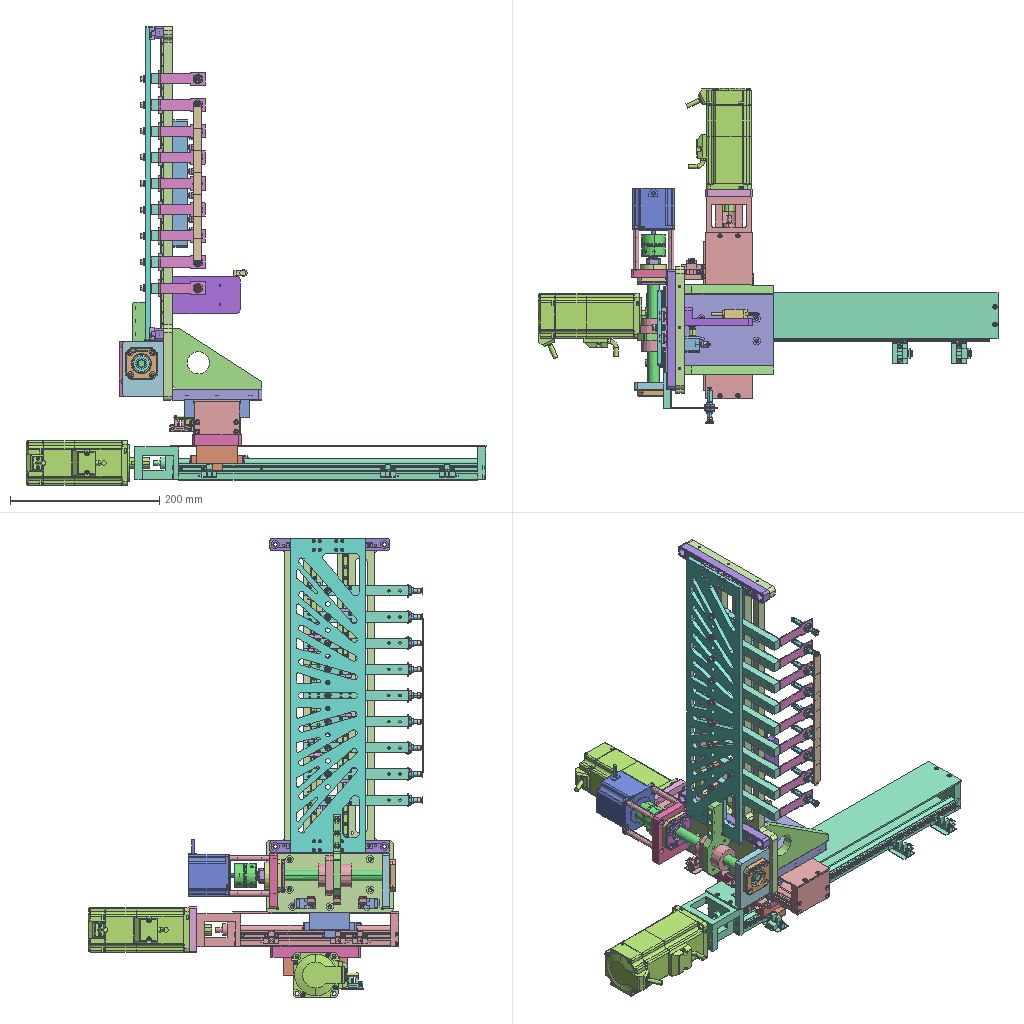Assembly | STEP file | 54 different items | 180 placed | box 616 x 450 x 614 mm
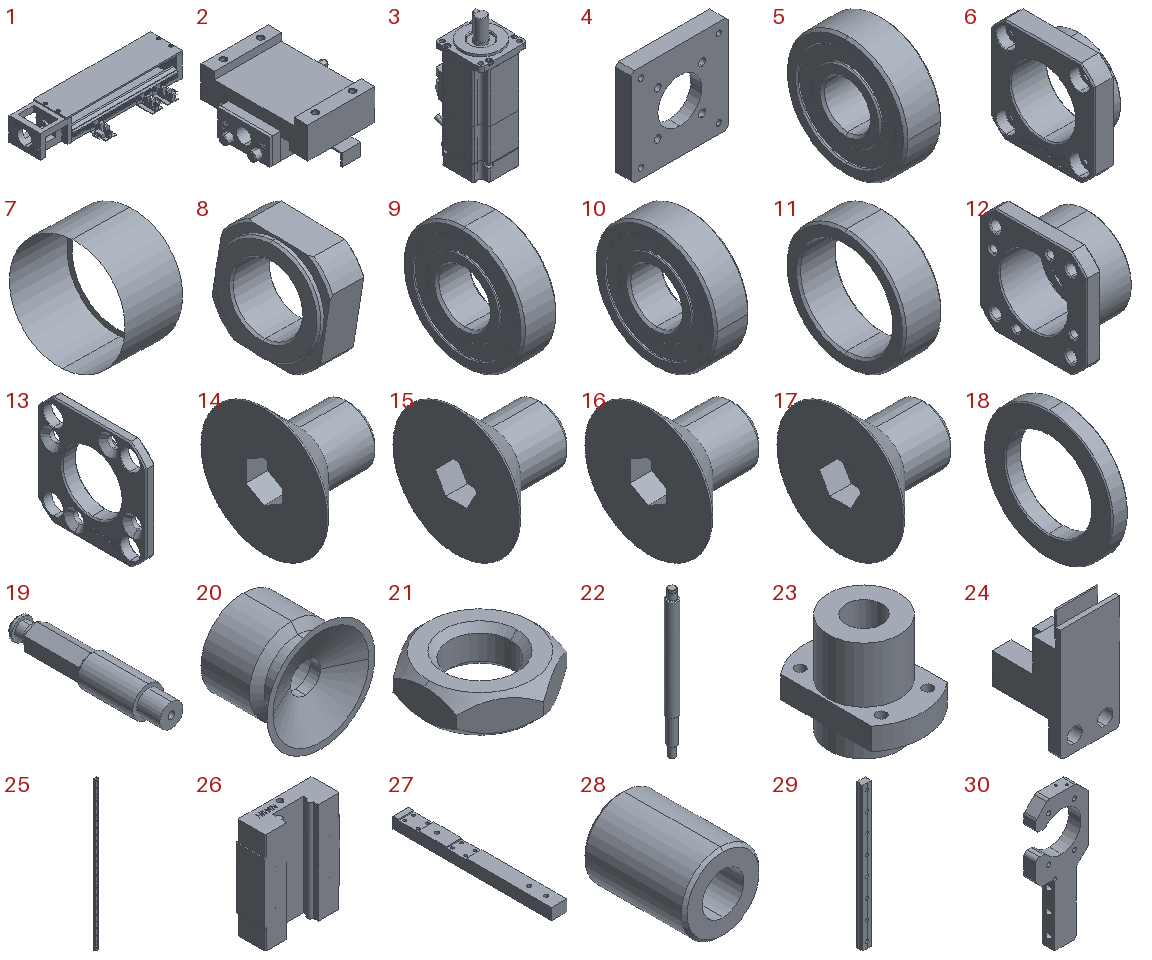Parts list (item | name | quantity | parent item | size | volume):
1 | PRODUCT_ID_1-C-F0-200 | x1 | in KK6005C-200A1-F0CS1-HiwinCorporation-07-20-2018 | 270.02 x 94.86 x 47 mm | 309343 mm3
2 | PRODUCT_ID_2-C-F0-200 | x1 | in KK6005C-200A1-F0CS1-HiwinCorporation-07-20-2018 | 83.5 x 94 x 36 mm | 123650 mm3
3 | C20604RS(Delta 400W) Servo Motor | x2 | in KK6005C-200A1-F0CS1-HiwinCorporation-07-20-2018, KK6010C-400A1-F0CS1-HiwinCorporation-07-20-2018 | 60 x 87.491 x 165.5 mm | 457978 mm3
4 | KK60-F2E KK60 200W Flange Adapter | x1 | in KK6005C-200A1-F0CS1-HiwinCorporation-07-20-2018 | 62 x 10 x 62 mm | 27303 mm3
5 | 6000ZZ-1 | x1 | in LKFF12 | 8 x 26 x 26 mm | 3377 mm3
6 | LFF12-1-1 | x1 | in LKFF12 | 15 x 42 x 42 mm | 10904 mm3
7 | Lock nut 19X8X12 | x1 | in 7 | - | -
8 | Lock nut 19X8X12-1 | x1 | in 7 | 10.153 x 20.245 x 20.375 mm | 1688 mm3
9 | 7001-1 | x1 | in LKFK12 | 8 x 28 x 28 mm | 3796 mm3
10 | 7001_1-1 | x1 | in LKFK12 | 8 x 28 x 28 mm | 3796 mm3
11 | Spacer ring 15-5-12-1 | x1 | in LKFK12 | 5 x 15.5 x 15.5 mm | 371.674 mm3
12 | LFK12-1 | x1 | in LKFK12 | 23 x 44 x 44 mm | 14384 mm3
13 | LFK12-MOD-1 | x1 | in LKFK12 | 6 x 44 x 44 mm | 4397 mm3
14 | M4-6-1 | x1 | in LKFK12 | 6 x 8.819 x 8.819 mm | 121.278 mm3
15 | M4-6_1-1 | x1 | in LKFK12 | 6 x 8.819 x 8.819 mm | 121.278 mm3
16 | M4-6_2-1 | x1 | in LKFK12 | 6 x 8.819 x 8.819 mm | 121.278 mm3
17 | M4-6_3-1 | x1 | in LKFK12 | 6 x 8.819 x 8.819 mm | 121.278 mm3
18 | Oil seal 24X3X16-1 | x1 | in LKFK12 | 3 x 24 x 24 mm | 748.955 mm3
19 | HI_WEJ41-d8-WEM11-K-6-U4-001 | x9 | in WEJ41-d8-WEM11-K-6-U4, WEJ41-d8-WEM11-K-6-U4-1, WEJ41-d8-WEM11-K-6-U4-2, WEJ41-d8-WEM11-K-6-U4-3, WEJ41-d8-WEM11-K-6-U4-4, WEJ41-d8-WEM11-K-6-U4-5, WEJ41-d8-WEM11-K-6-U4-6, WEJ41-d8-WEM11-K-6-U4-7, WEJ41-d8-WEM11-K-6-U4-8 | 8 x 40 x 8 mm | 1332 mm3
20 | HI_WEJ51-d8-WEM11-6-003 | x9 | in WEJ41-d8-WEM11-K-6-U4, WEJ41-d8-WEM11-K-6-U4-1, WEJ41-d8-WEM11-K-6-U4-2, WEJ41-d8-WEM11-K-6-U4-3, WEJ41-d8-WEM11-K-6-U4-4, WEJ41-d8-WEM11-K-6-U4-5, WEJ41-d8-WEM11-K-6-U4-6, WEJ41-d8-WEM11-K-6-U4-7, WEJ41-d8-WEM11-K-6-U4-8 | 9 x 6.5 x 9 mm | 149.71 mm3
21 | HI_WEJ41-d8-WEM11-K-6-U4-002 | x18 | in WEJ41-d8-WEM11-K-6-U4, WEJ41-d8-WEM11-K-6-U4-1, WEJ41-d8-WEM11-K-6-U4-2, WEJ41-d8-WEM11-K-6-U4-3, WEJ41-d8-WEM11-K-6-U4-4, WEJ41-d8-WEM11-K-6-U4-5, WEJ41-d8-WEM11-K-6-U4-6, WEJ41-d8-WEM11-K-6-U4-7, WEJ41-d8-WEM11-K-6-U4-8 | 12 x 13.856 x 4 mm | 327.385 mm3
22 | HI_LCP02-16-16-L200-F15-P8 | x1 | in LCP02-16-16-L200-F15-P8 | 15 x 15 x 200 mm | 29982 mm3
23 | HI_LCP02-16-16-L200-F15-P8_2 | x1 | in LCP02-16-16-L200-F15-P8 | 34 x 53 x 45 mm | 34960 mm3
24 | xgSENSOR(EE-SX674) | x2 | in PN_0001 Adjustable-Pitch Pick-up Nozzle | 13.6 x 15.5 x 27.3 mm | 2060 mm3
25 | MGN7C-Rail L385 | x2 | in PN_0001 Adjustable-Pitch Pick-up Nozzle | 7 x 4.8 x 385 mm | 11143 mm3
26 | MGN7C-Slider | x13 | in PN_0001 Adjustable-Pitch Pick-up Nozzle | 17 x 6.5 x 22.5 mm | 1844 mm3
27 | PN_0003 | x9 | in PN_0001 Adjustable-Pitch Pick-up Nozzle | 13.5 x 140 x 10 mm | 17518 mm3
28 | PN_0004 | x9 | in PN_0001 Adjustable-Pitch Pick-up Nozzle | 8 x 10.5 x 8 mm | 373.101 mm3
29 | MGN7C-Rail L115 | x2 | in PN_0001 Adjustable-Pitch Pick-up Nozzle | 7 x 4.8 x 115 mm | 3319 mm3
30 | PN_0007 | x1 | in PN_0001 Adjustable-Pitch Pick-up Nozzle | 43 x 10 x 110 mm | 21722 mm3
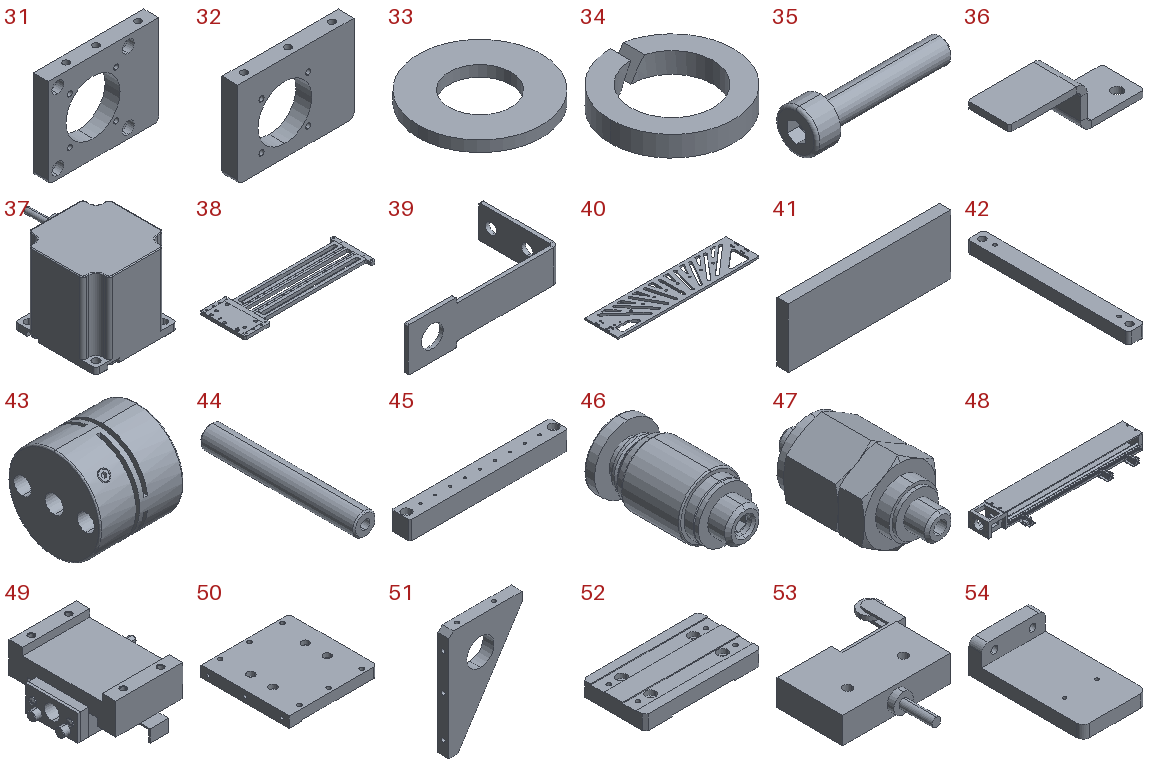31 | PN_0008 | x1 | in PN_0001 Adjustable-Pitch Pick-up Nozzle | 74 x 10 x 60 mm | 31735 mm3
32 | PN_0009 | x1 | in PN_0001 Adjustable-Pitch Pick-up Nozzle | 74 x 10 x 55 mm | 30537 mm3
33 | Plain Washer Grade C GB T 95-1985 4 | x9 | in PN_0001 Adjustable-Pitch Pick-up Nozzle | 9 x 9 x 0.8 mm | 38.17 mm3
34 | Spring Washer GB T 93-1987 4 | x9 | in PN_0001 Adjustable-Pitch Pick-up Nozzle | 6.6 x 6.6 x 1.1 mm | 20.135 mm3
35 | Socket Head Cap Screw GB T 70.1-2000 M4X20-C | x9 | in PN_0001 Adjustable-Pitch Pick-up Nozzle | 24 x 7 x 7 mm | 386.251 mm3
36 | PN_0010(Default) | x3 | in PN_0001 Adjustable-Pitch Pick-up Nozzle | 31.5 x 10 x 10 mm | 561.991 mm3
37 | HSTM57-1.8-S-56 | x1 | in PN_0001 Adjustable-Pitch Pick-up Nozzle | 56.438 x 76.419 x 75.6 mm | 160609 mm3
38 | PN_0005 | x1 | in PN_0001 Adjustable-Pitch Pick-up Nozzle | 500 x 170 x 12 mm | 536065 mm3
39 | PN_0011(Default) | x9 | in PN_0001 Adjustable-Pitch Pick-up Nozzle | 62.237 x 31.5 x 18 mm | 1846 mm3
40 | PN_0002 | x1 | in PN_0001 Adjustable-Pitch Pick-up Nozzle | 420 x 100 x 6 mm | 175315 mm3
41 | Part 29.58X10.85X2.08 | x7 | in PN_0001 Adjustable-Pitch Pick-up Nozzle | 29.58 x 2.08 x 10.85 mm | 667.561 mm3
42 | PN_0006a | x2 | in PN_0001 Adjustable-Pitch Pick-up Nozzle | 16 x 160 x 12 mm | 27789 mm3
43 | DBA01-D32-d6.35-e8 | x1 | in PN_0001 Adjustable-Pitch Pick-up Nozzle | 29 x 32 x 32 mm | 19412 mm3
44 | PN_0012 | x4 | in PN_0001 Adjustable-Pitch Pick-up Nozzle | 8 x 55 x 8 mm | 2556 mm3
45 | PN_0013 | x1 | in PN_0001 Adjustable-Pitch Pick-up Nozzle | 170 x 20 x 20 mm | 64184 mm3
46 | BPOC4M5 | x9 | in PN_0001 Adjustable-Pitch Pick-up Nozzle | 9.5 x 18.5 x 9.5 mm | 733.541 mm3
47 | BKC0425-M3 | x9 | in PN_0001 Adjustable-Pitch Pick-up Nozzle | 8 x 17 x 9.238 mm | 562.812 mm3
48 | PRODUCT_ID_1-C-F0-400 | x1 | in KK6010C-400A1-F0CS1-HiwinCorporation-07-20-2018 | 470.02 x 94.86 x 47 mm | 498801 mm3
49 | PRODUCT_ID_2-C-F0-400 | x1 | in KK6010C-400A1-F0CS1-HiwinCorporation-07-20-2018 | 83.5 x 94 x 36 mm | 123650 mm3
50 | PN_0014 | x1 | - | 120 x 120 x 15 mm | 192156 mm3
51 | PN_0015 | x2 | - | 81 x 12 x 120 mm | 60149 mm3
52 | PN_0016 | x1 | - | 120 x 65 x 15 mm | 102204 mm3
53 | Micro Switch ZIR52-1703 | x1 | - | 58.94 x 64.5 x 12 mm | 16845 mm3
54 | PN_0017 | x1 | - | 50 x 90 x 25 mm | 51712 mm3
Placements (level | parent | child | x y z in mm | rotation matrix by rows):
1 | subassembly 2 | KK6005C-200A1-F0CS1-HiwinCorporation-07-20-2018 | 51.0 100.0 60.5 | 0 1 0 -1 0 0 0 0 1
2 | KK6005C-200A1-F0CS1-HiwinCorporation-07-20-2018 | PRODUCT_ID_1-C-F0-200 | -0.0 -0.0 -0.0 | 1 0 0 0 1 0 0 0 1
2 | KK6005C-200A1-F0CS1-HiwinCorporation-07-20-2018 | PRODUCT_ID_2-C-F0-200 | 19.0 -0.0 -0.0 | 1 0 0 0 1 0 0 0 1
2 | KK6005C-200A1-F0CS1-HiwinCorporation-07-20-2018 | C20604RS(Delta 400W) Servo Motor | -66.0 -0.0 -0.0 | 0 0 1 0 -1 0 1 0 0
2 | KK6005C-200A1-F0CS1-HiwinCorporation-07-20-2018 | KK60-F2E KK60 200W Flange Adapter | -59.0 -0.0 -0.0 | 0 -1 0 1 0 0 0 0 1
1 | subassembly 2 | PN_0001 Adjustable-Pitch Pick-up Nozzle | -246.073 -225.56 374.0 | -1 0 0 0 1 0 0 0 -1
2 | PN_0001 Adjustable-Pitch Pick-up Nozzle | LKFF12 | -170.073 118.034 262.0 | 0 -1 0 1 0 0 0 0 1
3 | LKFF12 | 6000ZZ-1 | -0.0 0.0 -0.0 | 1 0 0 0 1 0 0 0 1
3 | LKFF12 | LFF12-1-1 | -0.0 0.0 -0.0 | 1 0 0 0 1 0 0 0 1
2 | PN_0001 Adjustable-Pitch Pick-up Nozzle | LKFK12 | -169.036 271.087 262.954 | 0 -1 0.00171 1 0 0 0 0.00171 1
3 | LKFK12 | Lock nut 19X8X12 | 22.348 43.346 2.499 | 0.9935 0.07258 -0.08741 -0.07258 0.9974 0.003182 0.08741 0.003182 0.9962
4 | Lock nut 19X8X12 | Lock nut 19X8X12 | -0.0 -0.0 -0.0 | 1 0 0 0 1 0 0 0 1
4 | Lock nut 19X8X12 | Lock nut 19X8X12-1 | -0.0 -0.0 -0.0 | 1 0 0 0 1 0 0 0 1
3 | LKFK12 | 7001-1 | -0.0 -0.0 0.0 | 1 0 0 0 1 0 0 0 1
3 | LKFK12 | 7001_1-1 | -0.0 -0.0 0.0 | 1 0 0 0 1 0 0 0 1
3 | LKFK12 | Spacer ring 15-5-12-1 | 6.641 -31.327 19.206 | 1 0 0 0 1 0 0 0 1
3 | LKFK12 | LFK12-1 | -0.0 -0.0 0.0 | 1 0 0 0 1 0 0 0 1
3 | LKFK12 | LFK12-MOD-1 | -0.0 -0.0 0.0 | 1 0 0 0 1 0 0 0 1
3 | LKFK12 | M4-6-1 | -0.0 -0.0 0.0 | 1 0 0 0 1 0 0 0 1
3 | LKFK12 | M4-6_1-1 | -0.0 -0.0 0.0 | 1 0 0 0 1 0 0 0 1
3 | LKFK12 | M4-6_2-1 | -0.0 -0.0 0.0 | 1 0 0 0 1 0 0 0 1
3 | LKFK12 | M4-6_3-1 | -0.0 -0.0 0.0 | 1 0 0 0 1 0 0 0 1
3 | LKFK12 | Oil seal 24X3X16-1 | -0.0 -0.0 0.0 | 1 0 0 0 1 0 0 0 1
2 | PN_0001 Adjustable-Pitch Pick-up Nozzle | WEJ41-d8-WEM11-K-6-U4 | -271.31 102.59 140.076 | 1 0 0 0 1 0 0 0 1
3 | WEJ41-d8-WEM11-K-6-U4 | HI_WEJ41-d8-WEM11-K-6-U4-001 | -0.0 -13.5 -0.0 | 1 0 0 0 1 0 0 0 1
3 | WEJ41-d8-WEM11-K-6-U4 | HI_WEJ51-d8-WEM11-6-003 | -0.0 -13.5 -0.0 | 1 0 0 0 1 0 0 0 1
3 | WEJ41-d8-WEM11-K-6-U4 | HI_WEJ41-d8-WEM11-K-6-U4-002 | 0.0 -1.5 0.0 | 1 0 0 0 0 -1 0 1 0
3 | WEJ41-d8-WEM11-K-6-U4 | HI_WEJ41-d8-WEM11-K-6-U4-002 | 0.0 -0.0 0.0 | 1 0 0 0 0 1 0 -1 0
2 | PN_0001 Adjustable-Pitch Pick-up Nozzle | WEJ41-d8-WEM11-K-6-U4-1 | -271.31 102.59 105.066 | 1 0 0 0 1 0 0 0 1
3 | WEJ41-d8-WEM11-K-6-U4-1 | HI_WEJ41-d8-WEM11-K-6-U4-001 | -0.0 -13.5 0.0 | 1 0 0 0 1 0 0 0 1
3 | WEJ41-d8-WEM11-K-6-U4-1 | HI_WEJ51-d8-WEM11-6-003 | -0.0 -13.5 0.0 | 1 0 0 0 1 0 0 0 1
3 | WEJ41-d8-WEM11-K-6-U4-1 | HI_WEJ41-d8-WEM11-K-6-U4-002 | 0.0 -1.5 0.0 | 1 0 0 0 0 -1 0 1 0
3 | WEJ41-d8-WEM11-K-6-U4-1 | HI_WEJ41-d8-WEM11-K-6-U4-002 | 0.0 -0.0 0.0 | 1 0 0 0 0 1 0 -1 0
2 | PN_0001 Adjustable-Pitch Pick-up Nozzle | WEJ41-d8-WEM11-K-6-U4-2 | -271.31 102.59 70.058 | 1 0 0 0 1 0 0 0 1
3 | WEJ41-d8-WEM11-K-6-U4-2 | HI_WEJ41-d8-WEM11-K-6-U4-001 | -0.0 -13.5 0.0 | 1 0 0 0 1 0 0 0 1
3 | WEJ41-d8-WEM11-K-6-U4-2 | HI_WEJ51-d8-WEM11-6-003 | -0.0 -13.5 0.0 | 1 0 0 0 1 0 0 0 1
3 | WEJ41-d8-WEM11-K-6-U4-2 | HI_WEJ41-d8-WEM11-K-6-U4-002 | 0.0 -1.5 0.0 | 1 0 0 0 0 -1 0 1 0
3 | WEJ41-d8-WEM11-K-6-U4-2 | HI_WEJ41-d8-WEM11-K-6-U4-002 | 0.0 -0.0 0.0 | 1 0 0 0 0 1 0 -1 0
2 | PN_0001 Adjustable-Pitch Pick-up Nozzle | WEJ41-d8-WEM11-K-6-U4-3 | -271.31 102.59 35.052 | 1 0 0 0 1 0 0 0 1
3 | WEJ41-d8-WEM11-K-6-U4-3 | HI_WEJ41-d8-WEM11-K-6-U4-001 | -0.0 -13.5 0.0 | 1 0 0 0 1 0 0 0 1
3 | WEJ41-d8-WEM11-K-6-U4-3 | HI_WEJ51-d8-WEM11-6-003 | -0.0 -13.5 0.0 | 1 0 0 0 1 0 0 0 1
3 | WEJ41-d8-WEM11-K-6-U4-3 | HI_WEJ41-d8-WEM11-K-6-U4-002 | 0.0 -1.5 0.0 | 1 0 0 0 0 -1 0 1 0
3 | WEJ41-d8-WEM11-K-6-U4-3 | HI_WEJ41-d8-WEM11-K-6-U4-002 | 0.0 -0.0 0.0 | 1 0 0 0 0 1 0 -1 0
2 | PN_0001 Adjustable-Pitch Pick-up Nozzle | WEJ41-d8-WEM11-K-6-U4-4 | -271.31 102.59 0.0 | -0.07822 0 0.9969 0 1 0 -0.9969 0 -0.07822
3 | WEJ41-d8-WEM11-K-6-U4-4 | HI_WEJ41-d8-WEM11-K-6-U4-001 | -0.0 -13.5 -0.0 | 1 0 0 0 1 0 0 0 1
3 | WEJ41-d8-WEM11-K-6-U4-4 | HI_WEJ51-d8-WEM11-6-003 | -0.0 -13.5 -0.0 | 1 0 0 0 1 0 0 0 1
3 | WEJ41-d8-WEM11-K-6-U4-4 | HI_WEJ41-d8-WEM11-K-6-U4-002 | -0.0 -1.5 -0.0 | 1 0 0 0 0 -1 0 1 0
3 | WEJ41-d8-WEM11-K-6-U4-4 | HI_WEJ41-d8-WEM11-K-6-U4-002 | -0.0 -0.0 -0.0 | 1 0 0 0 0 1 0 -1 -0
2 | PN_0001 Adjustable-Pitch Pick-up Nozzle | WEJ41-d8-WEM11-K-6-U4-5 | -271.31 102.59 -35.052 | 1 0 0 0 1 0 0 0 1
3 | WEJ41-d8-WEM11-K-6-U4-5 | HI_WEJ41-d8-WEM11-K-6-U4-001 | -0.0 -13.5 0.0 | 1 0 0 0 1 0 0 0 1
3 | WEJ41-d8-WEM11-K-6-U4-5 | HI_WEJ51-d8-WEM11-6-003 | -0.0 -13.5 0.0 | 1 0 0 0 1 0 0 0 1
3 | WEJ41-d8-WEM11-K-6-U4-5 | HI_WEJ41-d8-WEM11-K-6-U4-002 | 0.0 -1.5 0.0 | 1 0 0 0 0 -1 0 1 0
3 | WEJ41-d8-WEM11-K-6-U4-5 | HI_WEJ41-d8-WEM11-K-6-U4-002 | 0.0 -0.0 0.0 | 1 0 0 0 0 1 0 -1 0
2 | PN_0001 Adjustable-Pitch Pick-up Nozzle | WEJ41-d8-WEM11-K-6-U4-6 | -271.31 102.59 -70.058 | 1 0 0 0 1 0 0 0 1
3 | WEJ41-d8-WEM11-K-6-U4-6 | HI_WEJ41-d8-WEM11-K-6-U4-001 | -0.0 -13.5 0.0 | 1 0 0 0 1 0 0 0 1
3 | WEJ41-d8-WEM11-K-6-U4-6 | HI_WEJ51-d8-WEM11-6-003 | -0.0 -13.5 0.0 | 1 0 0 0 1 0 0 0 1
3 | WEJ41-d8-WEM11-K-6-U4-6 | HI_WEJ41-d8-WEM11-K-6-U4-002 | 0.0 -1.5 0.0 | 1 0 0 0 0 -1 0 1 0
3 | WEJ41-d8-WEM11-K-6-U4-6 | HI_WEJ41-d8-WEM11-K-6-U4-002 | 0.0 -0.0 0.0 | 1 0 0 0 0 1 0 -1 0
2 | PN_0001 Adjustable-Pitch Pick-up Nozzle | WEJ41-d8-WEM11-K-6-U4-7 | -271.31 102.59 -140.076 | 0.9981 0 0.06111 0 1 0 -0.06111 0 0.9981
3 | WEJ41-d8-WEM11-K-6-U4-7 | HI_WEJ41-d8-WEM11-K-6-U4-001 | -0.0 -13.5 -0.0 | 1 0 0 0 1 0 0 0 1
3 | WEJ41-d8-WEM11-K-6-U4-7 | HI_WEJ51-d8-WEM11-6-003 | -0.0 -13.5 -0.0 | 1 0 0 0 1 0 0 0 1
3 | WEJ41-d8-WEM11-K-6-U4-7 | HI_WEJ41-d8-WEM11-K-6-U4-002 | -0.0 -1.5 -0.0 | 1 0 0 0 0 -1 0 1 0
3 | WEJ41-d8-WEM11-K-6-U4-7 | HI_WEJ41-d8-WEM11-K-6-U4-002 | -0.0 -0.0 -0.0 | 1 0 0 0 0 1 0 -1 -0
2 | PN_0001 Adjustable-Pitch Pick-up Nozzle | WEJ41-d8-WEM11-K-6-U4-8 | -271.31 102.59 -105.066 | 1 0 0 0 1 0 0 0 1
3 | WEJ41-d8-WEM11-K-6-U4-8 | HI_WEJ41-d8-WEM11-K-6-U4-001 | -0.0 -13.5 0.0 | 1 0 0 0 1 0 0 0 1
3 | WEJ41-d8-WEM11-K-6-U4-8 | HI_WEJ51-d8-WEM11-6-003 | -0.0 -13.5 0.0 | 1 0 0 0 1 0 0 0 1
3 | WEJ41-d8-WEM11-K-6-U4-8 | HI_WEJ41-d8-WEM11-K-6-U4-002 | 0.0 -1.5 0.0 | 1 0 0 0 0 -1 0 1 0
3 | WEJ41-d8-WEM11-K-6-U4-8 | HI_WEJ41-d8-WEM11-K-6-U4-002 | 0.0 -0.0 0.0 | 1 0 0 0 0 1 0 -1 0
2 | PN_0001 Adjustable-Pitch Pick-up Nozzle | LCP02-16-16-L200-F15-P8 | -196.073 118.493 241.0 | 1 0 0 0 0 -1 0 1 -0
3 | LCP02-16-16-L200-F15-P8 | HI_LCP02-16-16-L200-F15-P8 | -0.0 0.0 0.0 | 1 0 0 0 1 0 0 0 1
3 | LCP02-16-16-L200-F15-P8 | HI_LCP02-16-16-L200-F15-P8_2 | -0.0 0.0 0.0 | 1 0 0 0 1 0 0 0 1
2 | PN_0001 Adjustable-Pitch Pick-up Nozzle | xgSENSOR(EE-SX674) | -225.073 146.393 278.25 | 0 1 0 0 0 -1 -1 0 -0
2 | PN_0001 Adjustable-Pitch Pick-up Nozzle | xgSENSOR(EE-SX674) | -225.073 247.393 278.25 | 0 1 0 0 0 1 1 0 0
2 | PN_0001 Adjustable-Pitch Pick-up Nozzle | MGN7C-Rail L385 | -226.073 185.53 -172.5 | 0 1 0 -1 0 0 0 0 1
2 | PN_0001 Adjustable-Pitch Pick-up Nozzle | MGN7C-Rail L385 | -226.073 227.59 -172.5 | 0 1 0 -1 0 0 0 0 1
2 | PN_0001 Adjustable-Pitch Pick-up Nozzle | MGN7C-Slider | -214.573 224.04 201.0 | 0 1 0 0 0 -1 -1 0 -0
2 | PN_0001 Adjustable-Pitch Pick-up Nozzle | MGN7C-Slider | -226.073 227.59 -140.076 | 0 1 0 -1 0 0 0 0 1
2 | PN_0001 Adjustable-Pitch Pick-up Nozzle | MGN7C-Slider | -226.073 227.59 70.058 | 0 1 0 -1 0 0 0 0 1
2 | PN_0001 Adjustable-Pitch Pick-up Nozzle | MGN7C-Slider | -214.573 224.04 -201.0 | 0 1 0 0 0 -1 -1 0 -0
2 | PN_0001 Adjustable-Pitch Pick-up Nozzle | MGN7C-Slider | -214.573 194.04 201.0 | 0 1 0 0 0 -1 -1 0 -0
2 | PN_0001 Adjustable-Pitch Pick-up Nozzle | MGN7C-Slider | -226.073 227.59 140.076 | 0 1 0 -1 0 0 0 0 1
2 | PN_0001 Adjustable-Pitch Pick-up Nozzle | MGN7C-Slider | -214.573 194.04 -201.0 | 0 1 0 0 0 -1 -1 0 -0
2 | PN_0001 Adjustable-Pitch Pick-up Nozzle | MGN7C-Slider | -226.073 185.53 105.066 | 0 1 0 -1 0 0 0 0 1
2 | PN_0001 Adjustable-Pitch Pick-up Nozzle | MGN7C-Slider | -226.073 185.53 -105.066 | 0 1 0 -1 0 0 0 0 1
2 | PN_0001 Adjustable-Pitch Pick-up Nozzle | MGN7C-Slider | -226.073 185.53 35.052 | 0 1 0 -1 0 0 0 0 1
2 | PN_0001 Adjustable-Pitch Pick-up Nozzle | MGN7C-Slider | -226.073 185.53 -35.052 | 0 1 0 -1 0 0 0 0 1
2 | PN_0001 Adjustable-Pitch Pick-up Nozzle | MGN7C-Slider | -226.073 227.59 -0.0 | 0 1 0 -1 0 0 0 0 1
2 | PN_0001 Adjustable-Pitch Pick-up Nozzle | MGN7C-Slider | -226.073 227.59 -70.058 | 0 1 0 -1 0 0 0 0 1
2 | PN_0001 Adjustable-Pitch Pick-up Nozzle | PN_0003 | -214.073 171.09 -140.076 | 0 0 -1 0 1 0 1 0 0
2 | PN_0001 Adjustable-Pitch Pick-up Nozzle | PN_0003 | -214.073 171.09 35.052 | 0 0 -1 0 1 0 1 0 0
2 | PN_0001 Adjustable-Pitch Pick-up Nozzle | PN_0003 | -214.073 171.09 140.076 | 0 0 -1 0 1 0 1 0 0
2 | PN_0001 Adjustable-Pitch Pick-up Nozzle | PN_0003 | -214.073 171.09 -35.052 | 0 0 -1 0 1 0 1 0 0
2 | PN_0001 Adjustable-Pitch Pick-up Nozzle | PN_0003 | -214.073 171.09 -105.066 | 0 0 -1 0 1 0 1 0 0
2 | PN_0001 Adjustable-Pitch Pick-up Nozzle | PN_0003 | -214.073 171.09 70.058 | 0 0 -1 0 1 0 1 0 0
2 | PN_0001 Adjustable-Pitch Pick-up Nozzle | PN_0003 | -214.073 171.09 105.066 | 0 0 -1 0 1 0 1 0 0
2 | PN_0001 Adjustable-Pitch Pick-up Nozzle | PN_0003 | -214.073 171.09 -0.0 | 0 0 -1 0 1 0 1 0 0
2 | PN_0001 Adjustable-Pitch Pick-up Nozzle | PN_0003 | -214.073 171.09 -70.058 | 0 0 -1 0 1 0 1 0 0
2 | PN_0001 Adjustable-Pitch Pick-up Nozzle | PN_0004 | -205.323 209.04 -35.052 | 0 -1 0 -0.9888 0 -0.149 0.149 0 -0.9888
2 | PN_0001 Adjustable-Pitch Pick-up Nozzle | PN_0004 | -205.323 209.04 70.058 | 0 1 0 -0.201 0 0.9796 0.9796 0 0.201
2 | PN_0001 Adjustable-Pitch Pick-up Nozzle | PN_0004 | -205.323 209.04 35.052 | 0 1 0 -0.201 0 0.9796 0.9796 0 0.201
2 | PN_0001 Adjustable-Pitch Pick-up Nozzle | PN_0004 | -205.323 209.04 -0.0 | 0 1 0 -0.5153 0 0.857 0.857 0 0.5153
2 | PN_0001 Adjustable-Pitch Pick-up Nozzle | PN_0004 | -205.323 209.04 -70.058 | 0 1 0 -0.4151 0 0.9098 0.9098 0 0.4151
2 | PN_0001 Adjustable-Pitch Pick-up Nozzle | PN_0004 | -205.323 209.04 140.076 | 0 1 0 0.4098 0 -0.9122 -0.9122 0 -0.4098
2 | PN_0001 Adjustable-Pitch Pick-up Nozzle | PN_0004 | -205.323 209.04 -140.076 | 0 1 0 -0.5153 0 0.857 0.857 0 0.5153
2 | PN_0001 Adjustable-Pitch Pick-up Nozzle | PN_0004 | -205.323 209.04 105.066 | 0 1 0 0.8533 0 -0.5214 -0.5214 0 -0.8533
2 | PN_0001 Adjustable-Pitch Pick-up Nozzle | PN_0004 | -205.323 209.04 -105.066 | 0 1 0 -0.4151 0 0.9098 0.9098 0 0.4151
2 | PN_0001 Adjustable-Pitch Pick-up Nozzle | MGN7C-Rail L115 | -214.573 244.06 -201.0 | 0 1 0 0 0 -1 -1 0 -0
2 | PN_0001 Adjustable-Pitch Pick-up Nozzle | MGN7C-Rail L115 | -214.573 244.06 201.0 | 0 1 0 0 0 -1 -1 0 -0
2 | PN_0001 Adjustable-Pitch Pick-up Nozzle | PN_0007 | -196.073 201.893 241.0 | 1 0 0 0 1 0 0 0 1
2 | PN_0001 Adjustable-Pitch Pick-up Nozzle | PN_0008 | -196.073 277.087 248.0 | 0 0 -1 0 1 0 1 0 -0
2 | PN_0001 Adjustable-Pitch Pick-up Nozzle | PN_0009 | -198.573 126.034 248.0 | 0 0 -1 0 1 0 1 0 -0
2 | PN_0001 Adjustable-Pitch Pick-up Nozzle | Plain Washer Grade C GB T 95-1985 4 | -200.073 209.04 -105.066 | 0 0 -1 -0.7058 0.7084 0 0.7084 0.7058 0
2 | PN_0001 Adjustable-Pitch Pick-up Nozzle | Plain Washer Grade C GB T 95-1985 4 | -200.073 209.04 -70.058 | 0 0 -1 -0.7058 0.7084 0 0.7084 0.7058 -0
2 | PN_0001 Adjustable-Pitch Pick-up Nozzle | Plain Washer Grade C GB T 95-1985 4 | -200.073 209.04 -140.076 | 0 0 -1 -0.9242 -0.3818 0 -0.3818 0.9242 0
2 | PN_0001 Adjustable-Pitch Pick-up Nozzle | Plain Washer Grade C GB T 95-1985 4 | -200.073 209.04 -35.052 | 0 0 -1 -0.7058 0.7084 0 0.7084 0.7058 -0
2 | PN_0001 Adjustable-Pitch Pick-up Nozzle | Plain Washer Grade C GB T 95-1985 4 | -200.073 209.04 70.058 | 0 0 -1 0.7058 -0.7084 0 -0.7084 -0.7058 0
2 | PN_0001 Adjustable-Pitch Pick-up Nozzle | Plain Washer Grade C GB T 95-1985 4 | -199.273 209.04 140.076 | 0 0 1 0 1 0 -1 0 -0
2 | PN_0001 Adjustable-Pitch Pick-up Nozzle | Plain Washer Grade C GB T 95-1985 4 | -200.073 209.04 35.052 | 0 0 -1 -0.9242 -0.3818 0 -0.3818 0.9242 0
2 | PN_0001 Adjustable-Pitch Pick-up Nozzle | Plain Washer Grade C GB T 95-1985 4 | -200.073 209.04 0.0 | 0 0 -1 -0.7058 0.7084 0 0.7084 0.7058 0
2 | PN_0001 Adjustable-Pitch Pick-up Nozzle | Plain Washer Grade C GB T 95-1985 4 | -200.073 209.04 105.066 | 0 0 -1 -0.9242 -0.3818 0 -0.3818 0.9242 0
2 | PN_0001 Adjustable-Pitch Pick-up Nozzle | Spring Washer GB T 93-1987 4 | -199.273 209.04 -70.058 | 0 0 -1 -0.9882 -0.1529 0 -0.1529 0.9882 -0
2 | PN_0001 Adjustable-Pitch Pick-up Nozzle | Spring Washer GB T 93-1987 4 | -199.273 209.04 -140.076 | 0 0 -1 -0.236 -0.9718 0 -0.9718 0.236 0
2 | PN_0001 Adjustable-Pitch Pick-up Nozzle | Spring Washer GB T 93-1987 4 | -199.273 209.04 -35.052 | 0 0 -1 0.9242 0.3818 0 0.3818 -0.9242 0
2 | PN_0001 Adjustable-Pitch Pick-up Nozzle | Spring Washer GB T 93-1987 4 | -199.273 209.04 70.058 | 0 0 -1 0.9242 0.3818 0 0.3818 -0.9242 0
2 | PN_0001 Adjustable-Pitch Pick-up Nozzle | Spring Washer GB T 93-1987 4 | -199.273 209.04 35.052 | 0 0 -1 0.9242 0.3818 0 0.3818 -0.9242 0
2 | PN_0001 Adjustable-Pitch Pick-up Nozzle | Spring Washer GB T 93-1987 4 | -199.273 209.04 0.0 | 0 0 -1 0.9242 0.3818 0 0.3818 -0.9242 -0
2 | PN_0001 Adjustable-Pitch Pick-up Nozzle | Spring Washer GB T 93-1987 4 | -198.173 209.04 140.076 | 0 0 1 0 1 0 -1 0 -0
2 | PN_0001 Adjustable-Pitch Pick-up Nozzle | Spring Washer GB T 93-1987 4 | -199.273 209.04 105.066 | 0 0 -1 0 1 0 1 0 0
2 | PN_0001 Adjustable-Pitch Pick-up Nozzle | Spring Washer GB T 93-1987 4 | -199.273 209.04 -105.066 | 0 0 -1 -0.9882 -0.1529 0 -0.1529 0.9882 0
2 | PN_0001 Adjustable-Pitch Pick-up Nozzle | Socket Head Cap Screw GB T 70.1-2000 M4X20-C | -194.173 209.04 -140.076 | -1 0 0 0 -0.3818 0.9242 0 0.9242 0.3818
2 | PN_0001 Adjustable-Pitch Pick-up Nozzle | Socket Head Cap Screw GB T 70.1-2000 M4X20-C | -194.173 209.04 -35.052 | -1 0 0 0 0.9242 0.3818 0 0.3818 -0.9242
2 | PN_0001 Adjustable-Pitch Pick-up Nozzle | Socket Head Cap Screw GB T 70.1-2000 M4X20-C | -194.173 209.04 70.058 | -1 0 0 0 -0.3818 0.9242 0 0.9242 0.3818
2 | PN_0001 Adjustable-Pitch Pick-up Nozzle | Socket Head Cap Screw GB T 70.1-2000 M4X20-C | -194.173 209.04 35.052 | -1 0 0 0 -0.3818 0.9242 0 0.9242 0.3818
2 | PN_0001 Adjustable-Pitch Pick-up Nozzle | Socket Head Cap Screw GB T 70.1-2000 M4X20-C | -194.173 209.04 -0.0 | -1 0 0 0 -0.3818 0.9242 0 0.9242 0.3818
2 | PN_0001 Adjustable-Pitch Pick-up Nozzle | Socket Head Cap Screw GB T 70.1-2000 M4X20-C | -194.173 209.04 105.066 | -1 0 0 0 -0.7966 0.6046 0 0.6046 0.7966
2 | PN_0001 Adjustable-Pitch Pick-up Nozzle | Socket Head Cap Screw GB T 70.1-2000 M4X20-C | -194.173 209.04 -105.066 | -1 0 0 0 -0.9864 0.1646 0 0.1646 0.9864
2 | PN_0001 Adjustable-Pitch Pick-up Nozzle | Socket Head Cap Screw GB T 70.1-2000 M4X20-C | -194.173 209.04 -70.058 | -1 0 0 0 -0.9864 0.1646 0 0.1646 0.9864
2 | PN_0001 Adjustable-Pitch Pick-up Nozzle | Socket Head Cap Screw GB T 70.1-2000 M4X20-C | -194.173 209.04 140.076 | -1 0 0 0 -0.3818 0.9242 0 0.9242 0.3818
2 | PN_0001 Adjustable-Pitch Pick-up Nozzle | PN_0010(Default) | -200.073 161.893 270.5 | 1 0 0 0 1 0 0 0 1
2 | PN_0001 Adjustable-Pitch Pick-up Nozzle | PN_0010(Default) | -200.073 231.893 270.5 | 1 0 0 0 1 0 0 0 1
2 | PN_0001 Adjustable-Pitch Pick-up Nozzle | PN_0010(Default) | -200.073 196.893 270.5 | 1 0 0 0 1 0 0 0 1
2 | PN_0001 Adjustable-Pitch Pick-up Nozzle | HSTM57-1.8-S-56 | -196.073 356.087 241.0 | 1 0 0 0 0 1 0 -1 0
2 | PN_0001 Adjustable-Pitch Pick-up Nozzle | PN_0005 | -231.073 206.56 -0.0 | 0 0 1 0 1 0 -1 0 0
2 | PN_0001 Adjustable-Pitch Pick-up Nozzle | PN_0011(Default) | -251.31 102.59 70.058 | 1 0 0 0 1 0 0 0 1
2 | PN_0001 Adjustable-Pitch Pick-up Nozzle | PN_0011(Default) | -251.31 102.59 35.052 | 1 0 0 0 1 0 0 0 1
2 | PN_0001 Adjustable-Pitch Pick-up Nozzle | PN_0011(Default) | -251.31 102.59 -70.058 | 1 0 0 0 1 0 0 0 1
2 | PN_0001 Adjustable-Pitch Pick-up Nozzle | PN_0011(Default) | -251.31 102.59 0.0 | 1 0 0 0 1 0 0 0 1
2 | PN_0001 Adjustable-Pitch Pick-up Nozzle | PN_0011(Default) | -251.31 102.59 -140.076 | 1 0 0 0 1 0 0 0 1
2 | PN_0001 Adjustable-Pitch Pick-up Nozzle | PN_0011(Default) | -251.31 102.59 -105.066 | 1 0 0 0 1 0 0 0 1
2 | PN_0001 Adjustable-Pitch Pick-up Nozzle | PN_0011(Default) | -251.31 102.59 -35.052 | 1 0 0 0 1 0 0 0 1
2 | PN_0001 Adjustable-Pitch Pick-up Nozzle | PN_0011(Default) | -251.31 102.59 105.066 | 1 0 0 0 1 0 0 0 1
2 | PN_0001 Adjustable-Pitch Pick-up Nozzle | PN_0011(Default) | -251.31 102.59 140.076 | 1 0 0 0 1 0 0 0 1
2 | PN_0001 Adjustable-Pitch Pick-up Nozzle | PN_0002 | -204.573 209.04 0.0 | 0 0 1 0 1 0 -1 0 -0
2 | PN_0001 Adjustable-Pitch Pick-up Nozzle | Part 29.58X10.85X2.08 | -271.31 81.55 88.8 | 0 0 -1 0 1 0 1 0 0
2 | PN_0001 Adjustable-Pitch Pick-up Nozzle | Part 29.58X10.85X2.08 | -271.31 81.55 59.2 | 0 0 -1 0 1 0 1 0 0
2 | PN_0001 Adjustable-Pitch Pick-up Nozzle | Part 29.58X10.85X2.08 | -271.31 81.55 29.6 | 0 0 -1 0 1 0 1 0 0
2 | PN_0001 Adjustable-Pitch Pick-up Nozzle | Part 29.58X10.85X2.08 | -271.31 81.55 -0.0 | 0 0 -1 0 1 0 1 0 0
2 | PN_0001 Adjustable-Pitch Pick-up Nozzle | Part 29.58X10.85X2.08 | -271.31 81.55 -29.6 | 0 0 -1 0 1 0 1 0 0
2 | PN_0001 Adjustable-Pitch Pick-up Nozzle | Part 29.58X10.85X2.08 | -271.31 81.55 -59.2 | 0 0 -1 0 1 0 1 0 0
2 | PN_0001 Adjustable-Pitch Pick-up Nozzle | Part 29.58X10.85X2.08 | -271.31 81.55 -88.8 | 0 0 -1 0 1 0 1 0 0
2 | PN_0001 Adjustable-Pitch Pick-up Nozzle | PN_0006a | -220.073 206.56 -202.0 | 0 0 -1 0 1 0 1 0 -0
2 | PN_0001 Adjustable-Pitch Pick-up Nozzle | PN_0006a | -220.073 206.56 202.0 | 0 0 -1 0 -1 0 -1 0 -0
2 | PN_0001 Adjustable-Pitch Pick-up Nozzle | DBA01-D32-d6.35-e8 | -196.073 319.687 241.0 | 0 0.9985 0.05439 -1 0 0 0 -0.05439 0.9985
2 | PN_0001 Adjustable-Pitch Pick-up Nozzle | PN_0012 | -219.645 313.587 264.571 | 1 0 0 0 1 0 0 0 1
2 | PN_0001 Adjustable-Pitch Pick-up Nozzle | PN_0012 | -172.503 313.587 217.43 | 1 0 0 0 1 0 0 0 1
2 | PN_0001 Adjustable-Pitch Pick-up Nozzle | PN_0012 | -219.643 313.587 217.43 | 1 0 0 0 1 0 0 0 1
2 | PN_0001 Adjustable-Pitch Pick-up Nozzle | PN_0012 | -172.503 313.587 264.57 | 1 0 0 0 1 0 0 0 1
2 | PN_0001 Adjustable-Pitch Pick-up Nozzle | PN_0013 | -248.073 186.56 -0.0 | 0 0 -1 0 1 0 1 0 -0
2 | PN_0001 Adjustable-Pitch Pick-up Nozzle | BPOC4M5 | -248.073 193.66 -48.0 | 1 0 0 0 1 0 0 0 1
2 | PN_0001 Adjustable-Pitch Pick-up Nozzle | BPOC4M5 | -248.073 193.66 -32.0 | 1 0 0 0 1 0 0 0 1
2 | PN_0001 Adjustable-Pitch Pick-up Nozzle | BPOC4M5 | -248.073 193.66 -16.0 | 1 0 0 0 1 0 0 0 1
2 | PN_0001 Adjustable-Pitch Pick-up Nozzle | BPOC4M5 | -248.073 193.66 -64.0 | 1 0 0 0 1 0 0 0 1
2 | PN_0001 Adjustable-Pitch Pick-up Nozzle | BPOC4M5 | -248.073 193.66 -0.0 | 1 0 0 0 1 0 0 0 1
2 | PN_0001 Adjustable-Pitch Pick-up Nozzle | BPOC4M5 | -248.073 193.66 16.0 | 1 0 0 0 1 0 0 0 1
2 | PN_0001 Adjustable-Pitch Pick-up Nozzle | BPOC4M5 | -248.073 193.66 32.0 | 1 0 0 0 1 0 0 0 1
2 | PN_0001 Adjustable-Pitch Pick-up Nozzle | BPOC4M5 | -248.073 193.66 48.0 | 1 0 0 0 1 0 0 0 1
2 | PN_0001 Adjustable-Pitch Pick-up Nozzle | BPOC4M5 | -248.073 193.66 64.0 | 1 0 0 0 1 0 0 0 1
2 | PN_0001 Adjustable-Pitch Pick-up Nozzle | BKC0425-M3 | -255.473 186.56 32.0 | 0 -1 0 -0.3818 0 -0.9242 0.9242 0 -0.3818
2 | PN_0001 Adjustable-Pitch Pick-up Nozzle | BKC0425-M3 | -255.473 186.56 -64.0 | 0 -1 0 -0.3818 0 -0.9242 0.9242 0 -0.3818
2 | PN_0001 Adjustable-Pitch Pick-up Nozzle | BKC0425-M3 | -255.473 186.56 -48.0 | 0 -1 0 -0.3818 0 -0.9242 0.9242 0 -0.3818
2 | PN_0001 Adjustable-Pitch Pick-up Nozzle | BKC0425-M3 | -255.473 186.56 -32.0 | 0 -1 0 -0.3818 0 -0.9242 0.9242 0 -0.3818
2 | PN_0001 Adjustable-Pitch Pick-up Nozzle | BKC0425-M3 | -255.473 186.56 48.0 | 0 -1 0 -0.3818 0 -0.9242 0.9242 0 -0.3818
2 | PN_0001 Adjustable-Pitch Pick-up Nozzle | BKC0425-M3 | -255.473 186.56 -16.0 | 0 -1 0 -0.3818 0 -0.9242 0.9242 0 -0.3818
2 | PN_0001 Adjustable-Pitch Pick-up Nozzle | BKC0425-M3 | -255.473 186.56 64.0 | 0 -1 0 -0.3818 0 -0.9242 0.9242 0 -0.3818
2 | PN_0001 Adjustable-Pitch Pick-up Nozzle | BKC0425-M3 | -255.473 186.56 -0.0 | 0 -1 0 -0.3818 0 -0.9242 0.9242 0 -0.3818
2 | PN_0001 Adjustable-Pitch Pick-up Nozzle | BKC0425-M3 | -255.473 186.56 16.0 | 0 -1 0 -0.3818 0 -0.9242 0.9242 0 -0.3818
1 | subassembly 2 | KK6010C-400A1-F0CS1-HiwinCorporation-07-20-2018 | -0.0 -0.0 -0.0 | 1 0 0 0 1 0 0 0 1
2 | KK6010C-400A1-F0CS1-HiwinCorporation-07-20-2018 | C20604RS(Delta 400W) Servo Motor | -66.0 -0.0 -0.0 | 0 0 1 0 -1 0 1 0 0
2 | KK6010C-400A1-F0CS1-HiwinCorporation-07-20-2018 | PRODUCT_ID_1-C-F0-400 | -0.0 -0.0 -0.0 | 1 0 0 0 1 0 0 0 1
2 | KK6010C-400A1-F0CS1-HiwinCorporation-07-20-2018 | PRODUCT_ID_2-C-F0-400 | -149.0 -0.0 -0.0 | 1 0 0 0 1 0 0 0 1
1 | subassembly 2 | PN_0014 | 51.0 -19.0 84.0 | 1 0 0 0 1 0 0 0 1
1 | subassembly 2 | PN_0015 | -9.0 35.0 99.0 | 0 0 -1 0 1 0 1 0 -0
1 | subassembly 2 | PN_0015 | -9.0 -73.0 99.0 | 0 0 -1 0 1 0 1 0 -0
1 | subassembly 2 | PN_0016 | 51.0 -0.0 23.5 | 0 1 0 -1 0 0 0 0 1
1 | subassembly 2 | Micro Switch ZIR52-1703 | 45.2 2.265 200.4 | 0 1 0 0 0 1 1 0 -0
1 | subassembly 2 | PN_0017 | 82.0 -8.735 225.0 | 0 -1 0 0 0 1 -1 0 -0